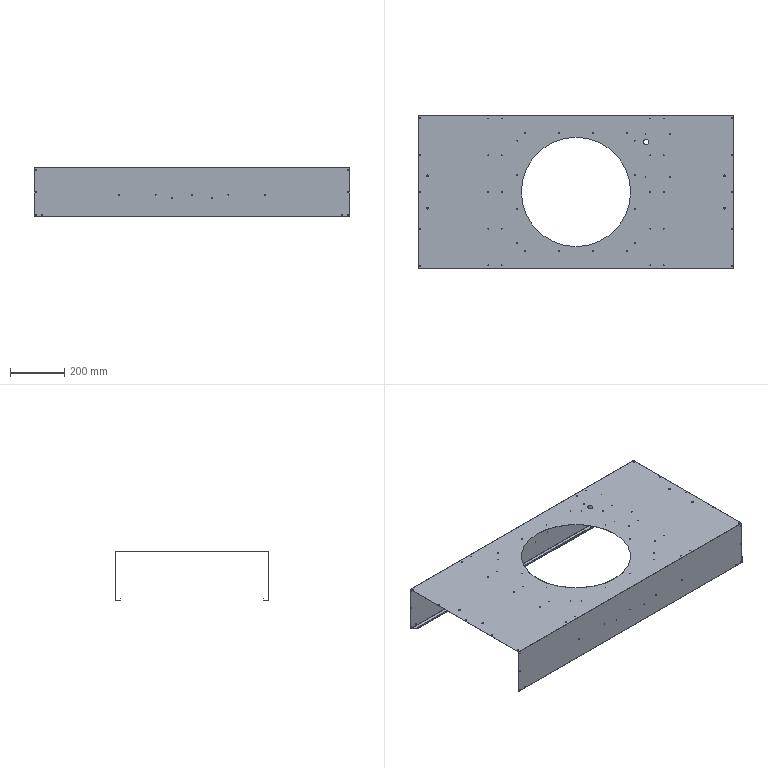Part | SolidWorks | features BaseBody 1 | 1 solid | 218 faces | box 1169 x 570 x 180 mm | volume 606575 mm3 | cylinder 184 | plane 30 | spline 4 | commonest cylinder face diameters 3.5 x120 2.7 x32 2.8 x8 6.5 x8 0.4 x6 1.6 x6